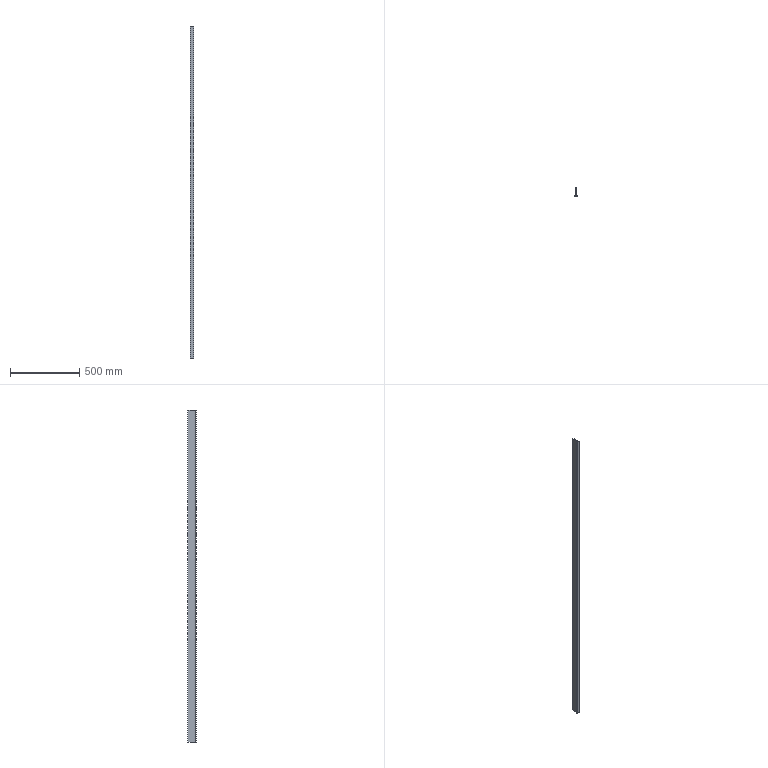Part | SolidWorks | features Fillet 2, Extrusion 1 | 1 solid | 12 faces | box 26 x 60 x 2400 mm | volume 1150265 mm3 | plane 8 | cylinder 4 | commonest cylinder face diameters 10 x2 16 x2
STEP:
#1=CARTESIAN_POINT('',(-3.,30.,0.));
#2=VERTEX_POINT('',#1);
#3=CARTESIAN_POINT('',(-3.,-17.,0.));
#4=VERTEX_POINT('',#3);
#5=CARTESIAN_POINT('',(-3.,30.,0.));
#6=DIRECTION('',(0.,-1.,0.));
#7=VECTOR('',#6,1000.);
#8=LINE('',#5,#7);
#9=EDGE_CURVE('',#2,#4,#8,.T.);
#10=ORIENTED_EDGE('',*,*,#9,.T.);
#11=CARTESIAN_POINT('',(-3.,-17.,2400.));
#12=VERTEX_POINT('',#11);
#13=CARTESIAN_POINT('',(-3.,-17.,2400.));
#14=DIRECTION('',(0.,0.,1.));
#15=VECTOR('',#14,1000.);
#16=LINE('',#13,#15);
#17=EDGE_CURVE('',#4,#12,#16,.T.);
#18=ORIENTED_EDGE('',*,*,#17,.T.);
#19=CARTESIAN_POINT('',(-3.,30.,2400.));
#20=VERTEX_POINT('',#19);
#21=CARTESIAN_POINT('',(-3.,30.,2400.));
#22=DIRECTION('',(0.,-1.,0.));
#23=VECTOR('',#22,1000.);
#24=LINE('',#21,#23);
#25=EDGE_CURVE('',#20,#12,#24,.T.);
#26=ORIENTED_EDGE('',*,*,#25,.F.);
#27=CARTESIAN_POINT('',(-3.,30.,2400.));
#28=DIRECTION('',(0.,0.,-1.));
#29=VECTOR('',#28,1000.);
#30=LINE('',#27,#29);
#31=EDGE_CURVE('',#20,#2,#30,.T.);
#32=ORIENTED_EDGE('',*,*,#31,.T.);
#33=EDGE_LOOP('',(#10,#18,#26,#32));
#34=FACE_OUTER_BOUND('',#33,.T.);
#35=CARTESIAN_POINT('',(-3.,30.,2400.));
#36=DIRECTION('',(1.,0.,0.));
#37=DIRECTION('',(0.,1.,0.));
#38=AXIS2_PLACEMENT_3D('',#35,#36,#37);
#39=PLANE('',#38);
#40=ADVANCED_FACE('',(#34),#39,.F.);
#41=CARTESIAN_POINT('',(-13.,-29.649,2400.));
#42=VERTEX_POINT('',#41);
#43=CARTESIAN_POINT('',(-13.,-30.,2400.));
#44=VERTEX_POINT('',#43);
#45=CARTESIAN_POINT('',(-13.,-25.,2400.));
#46=DIRECTION('',(0.,-1.,0.));
#47=VECTOR('',#46,1000.);
#48=LINE('',#45,#47);
#49=EDGE_CURVE('',#42,#44,#48,.T.);
#50=ORIENTED_EDGE('',*,*,#49,.F.);
#51=CARTESIAN_POINT('',(-13.,-29.649,0.));
#52=VERTEX_POINT('',#51);
#53=CARTESIAN_POINT('',(-13.,-29.649,2400.));
#54=DIRECTION('',(0.,0.,-1.));
#55=VECTOR('',#54,1000.);
#56=LINE('',#53,#55);
#57=EDGE_CURVE('',#42,#52,#56,.T.);
#58=ORIENTED_EDGE('',*,*,#57,.T.);
#59=CARTESIAN_POINT('',(-13.,-30.,0.));
#60=VERTEX_POINT('',#59);
#61=CARTESIAN_POINT('',(-13.,-25.,0.));
#62=DIRECTION('',(0.,-1.,0.));
#63=VECTOR('',#62,1000.);
#64=LINE('',#61,#63);
#65=EDGE_CURVE('',#52,#60,#64,.T.);
#66=ORIENTED_EDGE('',*,*,#65,.T.);
#67=CARTESIAN_POINT('',(-13.,-30.,2400.));
#68=DIRECTION('',(0.,0.,-1.));
#69=VECTOR('',#68,1000.);
#70=LINE('',#67,#69);
#71=EDGE_CURVE('',#44,#60,#70,.T.);
#72=ORIENTED_EDGE('',*,*,#71,.F.);
#73=EDGE_LOOP('',(#50,#58,#66,#72));
#74=FACE_OUTER_BOUND('',#73,.T.);
#75=CARTESIAN_POINT('',(-13.,-25.,2400.));
#76=DIRECTION('',(1.,0.,0.));
#77=DIRECTION('',(0.,0.,-1.));
#78=AXIS2_PLACEMENT_3D('',#75,#76,#77);
#79=PLANE('',#78);
#80=ADVANCED_FACE('',(#74),#79,.F.);
#81=CARTESIAN_POINT('',(13.,-30.,0.));
#82=VERTEX_POINT('',#81);
#83=CARTESIAN_POINT('',(-13.,-30.,0.));
#84=DIRECTION('',(1.,0.,0.));
#85=VECTOR('',#84,1000.);
#86=LINE('',#83,#85);
#87=EDGE_CURVE('',#60,#82,#86,.T.);
#88=ORIENTED_EDGE('',*,*,#87,.T.);
#89=CARTESIAN_POINT('',(13.,-30.,2400.));
#90=VERTEX_POINT('',#89);
#91=CARTESIAN_POINT('',(13.,-30.,2400.));
#92=DIRECTION('',(0.,0.,-1.));
#93=VECTOR('',#92,1000.);
#94=LINE('',#91,#93);
#95=EDGE_CURVE('',#90,#82,#94,.T.);
#96=ORIENTED_EDGE('',*,*,#95,.F.);
#97=CARTESIAN_POINT('',(-13.,-30.,2400.));
#98=DIRECTION('',(1.,0.,0.));
#99=VECTOR('',#98,1000.);
#100=LINE('',#97,#99);
#101=EDGE_CURVE('',#44,#90,#100,.T.);
#102=ORIENTED_EDGE('',*,*,#101,.F.);
#103=ORIENTED_EDGE('',*,*,#71,.T.);
#104=EDGE_LOOP('',(#88,#96,#102,#103));
#105=FACE_OUTER_BOUND('',#104,.T.);
#106=CARTESIAN_POINT('',(-13.,-30.,2400.));
#107=DIRECTION('',(0.,1.,0.));
#108=DIRECTION('',(0.,0.,1.));
#109=AXIS2_PLACEMENT_3D('',#106,#107,#108);
#110=PLANE('',#109);
#111=ADVANCED_FACE('',(#105),#110,.F.);
#112=CARTESIAN_POINT('',(13.,-29.649,0.));
#113=VERTEX_POINT('',#112);
#114=CARTESIAN_POINT('',(13.,-25.,0.));
#115=DIRECTION('',(0.,1.,0.));
#116=VECTOR('',#115,1000.);
#117=LINE('',#114,#116);
#118=EDGE_CURVE('',#82,#113,#117,.T.);
#119=ORIENTED_EDGE('',*,*,#118,.T.);
#120=CARTESIAN_POINT('',(13.,-29.649,2400.));
#121=VERTEX_POINT('',#120);
#122=CARTESIAN_POINT('',(13.,-29.649,2400.));
#123=DIRECTION('',(0.,0.,1.));
#124=VECTOR('',#123,1000.);
#125=LINE('',#122,#124);
#126=EDGE_CURVE('',#113,#121,#125,.T.);
#127=ORIENTED_EDGE('',*,*,#126,.T.);
#128=CARTESIAN_POINT('',(13.,-25.,2400.));
#129=DIRECTION('',(0.,1.,0.));
#130=VECTOR('',#129,1000.);
#131=LINE('',#128,#130);
#132=EDGE_CURVE('',#90,#121,#131,.T.);
#133=ORIENTED_EDGE('',*,*,#132,.F.);
#134=ORIENTED_EDGE('',*,*,#95,.T.);
#135=EDGE_LOOP('',(#119,#127,#133,#134));
#136=FACE_OUTER_BOUND('',#135,.T.);
#137=CARTESIAN_POINT('',(13.,-25.,2400.));
#138=DIRECTION('',(-1.,0.,0.));
#139=DIRECTION('',(0.,0.,1.));
#140=AXIS2_PLACEMENT_3D('',#137,#138,#139);
#141=PLANE('',#140);
#142=ADVANCED_FACE('',(#136),#141,.F.);
#143=CARTESIAN_POINT('',(3.,-17.,2400.));
#144=VERTEX_POINT('',#143);
#145=CARTESIAN_POINT('',(3.,30.,2400.));
#146=VERTEX_POINT('',#145);
#147=CARTESIAN_POINT('',(3.,30.,2400.));
#148=DIRECTION('',(0.,1.,0.));
#149=VECTOR('',#148,1000.);
#150=LINE('',#147,#149);
#151=EDGE_CURVE('',#144,#146,#150,.T.);
#152=ORIENTED_EDGE('',*,*,#151,.F.);
#153=CARTESIAN_POINT('',(3.,-17.,0.));
#154=VERTEX_POINT('',#153);
#155=CARTESIAN_POINT('',(3.,-17.,0.));
#156=DIRECTION('',(0.,0.,-1.));
#157=VECTOR('',#156,1000.);
#158=LINE('',#155,#157);
#159=EDGE_CURVE('',#144,#154,#158,.T.);
#160=ORIENTED_EDGE('',*,*,#159,.T.);
#161=CARTESIAN_POINT('',(3.,30.,0.));
#162=VERTEX_POINT('',#161);
#163=CARTESIAN_POINT('',(3.,30.,0.));
#164=DIRECTION('',(0.,1.,0.));
#165=VECTOR('',#164,1000.);
#166=LINE('',#163,#165);
#167=EDGE_CURVE('',#154,#162,#166,.T.);
#168=ORIENTED_EDGE('',*,*,#167,.T.);
#169=CARTESIAN_POINT('',(3.,30.,2400.));
#170=DIRECTION('',(0.,0.,-1.));
#171=VECTOR('',#170,1000.);
#172=LINE('',#169,#171);
#173=EDGE_CURVE('',#146,#162,#172,.T.);
#174=ORIENTED_EDGE('',*,*,#173,.F.);
#175=EDGE_LOOP('',(#152,#160,#168,#174));
#176=FACE_OUTER_BOUND('',#175,.T.);
#177=CARTESIAN_POINT('',(3.,30.,2400.));
#178=DIRECTION('',(-1.,0.,0.));
#179=DIRECTION('',(0.,-1.,0.));
#180=AXIS2_PLACEMENT_3D('',#177,#178,#179);
#181=PLANE('',#180);
#182=ADVANCED_FACE('',(#176),#181,.F.);
#183=CARTESIAN_POINT('',(-3.,30.,0.));
#184=DIRECTION('',(-1.,0.,0.));
#185=VECTOR('',#184,1000.);
#186=LINE('',#183,#185);
#187=EDGE_CURVE('',#162,#2,#186,.T.);
#188=ORIENTED_EDGE('',*,*,#187,.T.);
#189=ORIENTED_EDGE('',*,*,#31,.F.);
#190=CARTESIAN_POINT('',(-3.,30.,2400.));
#191=DIRECTION('',(-1.,0.,0.));
#192=VECTOR('',#191,1000.);
#193=LINE('',#190,#192);
#194=EDGE_CURVE('',#146,#20,#193,.T.);
#195=ORIENTED_EDGE('',*,*,#194,.F.);
#196=ORIENTED_EDGE('',*,*,#173,.T.);
#197=EDGE_LOOP('',(#188,#189,#195,#196));
#198=FACE_OUTER_BOUND('',#197,.T.);
#199=CARTESIAN_POINT('',(-3.,30.,2400.));
#200=DIRECTION('',(0.,-1.,0.));
#201=DIRECTION('',(0.,0.,-1.));
#202=AXIS2_PLACEMENT_3D('',#199,#200,#201);
#203=PLANE('',#202);
#204=ADVANCED_FACE('',(#198),#203,.F.);
#205=CARTESIAN_POINT('',(-9.154,-24.784,2400.));
#206=VERTEX_POINT('',#205);
#207=CARTESIAN_POINT('',(-11.,-17.,2400.));
#208=DIRECTION('',(0.,0.,-1.));
#209=DIRECTION('',(-1.,0.,0.));
#210=AXIS2_PLACEMENT_3D('',#207,#208,#209);
#211=CIRCLE('',#210,8.);
#212=EDGE_CURVE('',#12,#206,#211,.T.);
#213=ORIENTED_EDGE('',*,*,#212,.T.);
#214=CARTESIAN_POINT('',(-8.,-29.649,2400.));
#215=DIRECTION('',(0.,0.,1.));
#216=DIRECTION('',(-1.,0.,0.));
#217=AXIS2_PLACEMENT_3D('',#214,#215,#216);
#218=CIRCLE('',#217,5.);
#219=EDGE_CURVE('',#206,#42,#218,.T.);
#220=ORIENTED_EDGE('',*,*,#219,.T.);
#221=ORIENTED_EDGE('',*,*,#49,.T.);
#222=ORIENTED_EDGE('',*,*,#101,.T.);
#223=ORIENTED_EDGE('',*,*,#132,.T.);
#224=CARTESIAN_POINT('',(9.154,-24.784,2400.));
#225=VERTEX_POINT('',#224);
#226=CARTESIAN_POINT('',(8.,-29.649,2400.));
#227=DIRECTION('',(0.,0.,1.));
#228=DIRECTION('',(-1.,0.,0.));
#229=AXIS2_PLACEMENT_3D('',#226,#227,#228);
#230=CIRCLE('',#229,5.);
#231=EDGE_CURVE('',#121,#225,#230,.T.);
#232=ORIENTED_EDGE('',*,*,#231,.T.);
#233=CARTESIAN_POINT('',(11.,-17.,2400.));
#234=DIRECTION('',(0.,0.,-1.));
#235=DIRECTION('',(-1.,0.,0.));
#236=AXIS2_PLACEMENT_3D('',#233,#234,#235);
#237=CIRCLE('',#236,8.);
#238=EDGE_CURVE('',#225,#144,#237,.T.);
#239=ORIENTED_EDGE('',*,*,#238,.T.);
#240=ORIENTED_EDGE('',*,*,#151,.T.);
#241=ORIENTED_EDGE('',*,*,#194,.T.);
#242=ORIENTED_EDGE('',*,*,#25,.T.);
#243=EDGE_LOOP('',(#213,#220,#221,#222,#223,#232,#239,#240,#241,#242));
#244=FACE_OUTER_BOUND('',#243,.T.);
#245=CARTESIAN_POINT('',(-3.,-25.,2400.));
#246=DIRECTION('',(0.,0.,-1.));
#247=DIRECTION('',(-1.,0.,0.));
#248=AXIS2_PLACEMENT_3D('',#245,#246,#247);
#249=PLANE('',#248);
#250=ADVANCED_FACE('',(#244),#249,.F.);
#251=ORIENTED_EDGE('',*,*,#65,.F.);
#252=CARTESIAN_POINT('',(-9.154,-24.784,0.));
#253=VERTEX_POINT('',#252);
#254=CARTESIAN_POINT('',(-8.,-29.649,0.));
#255=DIRECTION('',(0.,0.,-1.));
#256=DIRECTION('',(-1.,0.,0.));
#257=AXIS2_PLACEMENT_3D('',#254,#255,#256);
#258=CIRCLE('',#257,5.);
#259=EDGE_CURVE('',#52,#253,#258,.T.);
#260=ORIENTED_EDGE('',*,*,#259,.T.);
#261=CARTESIAN_POINT('',(-11.,-17.,0.));
#262=DIRECTION('',(0.,0.,1.));
#263=DIRECTION('',(-1.,0.,0.));
#264=AXIS2_PLACEMENT_3D('',#261,#262,#263);
#265=CIRCLE('',#264,8.);
#266=EDGE_CURVE('',#253,#4,#265,.T.);
#267=ORIENTED_EDGE('',*,*,#266,.T.);
#268=ORIENTED_EDGE('',*,*,#9,.F.);
#269=ORIENTED_EDGE('',*,*,#187,.F.);
#270=ORIENTED_EDGE('',*,*,#167,.F.);
#271=CARTESIAN_POINT('',(9.154,-24.784,0.));
#272=VERTEX_POINT('',#271);
#273=CARTESIAN_POINT('',(11.,-17.,0.));
#274=DIRECTION('',(0.,0.,1.));
#275=DIRECTION('',(-1.,0.,0.));
#276=AXIS2_PLACEMENT_3D('',#273,#274,#275);
#277=CIRCLE('',#276,8.);
#278=EDGE_CURVE('',#154,#272,#277,.T.);
#279=ORIENTED_EDGE('',*,*,#278,.T.);
#280=CARTESIAN_POINT('',(8.,-29.649,0.));
#281=DIRECTION('',(0.,0.,-1.));
#282=DIRECTION('',(-1.,0.,0.));
#283=AXIS2_PLACEMENT_3D('',#280,#281,#282);
#284=CIRCLE('',#283,5.);
#285=EDGE_CURVE('',#272,#113,#284,.T.);
#286=ORIENTED_EDGE('',*,*,#285,.T.);
#287=ORIENTED_EDGE('',*,*,#118,.F.);
#288=ORIENTED_EDGE('',*,*,#87,.F.);
#289=EDGE_LOOP('',(#251,#260,#267,#268,#269,#270,#279,#286,#287,#288));
#290=FACE_OUTER_BOUND('',#289,.T.);
#291=CARTESIAN_POINT('',(-3.,-25.,0.));
#292=DIRECTION('',(0.,0.,-1.));
#293=DIRECTION('',(-1.,0.,0.));
#294=AXIS2_PLACEMENT_3D('',#291,#292,#293);
#295=PLANE('',#294);
#296=ADVANCED_FACE('',(#290),#295,.T.);
#297=ORIENTED_EDGE('',*,*,#266,.F.);
#298=CARTESIAN_POINT('',(-9.154,-24.784,2400.));
#299=DIRECTION('',(0.,0.,1.));
#300=VECTOR('',#299,1000.);
#301=LINE('',#298,#300);
#302=EDGE_CURVE('',#253,#206,#301,.T.);
#303=ORIENTED_EDGE('',*,*,#302,.T.);
#304=ORIENTED_EDGE('',*,*,#212,.F.);
#305=ORIENTED_EDGE('',*,*,#17,.F.);
#306=EDGE_LOOP('',(#297,#303,#304,#305));
#307=FACE_OUTER_BOUND('',#306,.T.);
#308=CARTESIAN_POINT('',(-11.,-17.,2400.));
#309=DIRECTION('',(0.,0.,1.));
#310=DIRECTION('',(1.,0.,0.));
#311=AXIS2_PLACEMENT_3D('',#308,#309,#310);
#312=CYLINDRICAL_SURFACE('',#311,8.);
#313=ADVANCED_FACE('',(#307),#312,.F.);
#314=ORIENTED_EDGE('',*,*,#238,.F.);
#315=CARTESIAN_POINT('',(9.154,-24.784,2400.));
#316=DIRECTION('',(0.,0.,-1.));
#317=VECTOR('',#316,1000.);
#318=LINE('',#315,#317);
#319=EDGE_CURVE('',#225,#272,#318,.T.);
#320=ORIENTED_EDGE('',*,*,#319,.T.);
#321=ORIENTED_EDGE('',*,*,#278,.F.);
#322=ORIENTED_EDGE('',*,*,#159,.F.);
#323=EDGE_LOOP('',(#314,#320,#321,#322));
#324=FACE_OUTER_BOUND('',#323,.T.);
#325=CARTESIAN_POINT('',(11.,-17.,2400.));
#326=DIRECTION('',(0.,0.,1.));
#327=DIRECTION('',(1.,0.,0.));
#328=AXIS2_PLACEMENT_3D('',#325,#326,#327);
#329=CYLINDRICAL_SURFACE('',#328,8.);
#330=ADVANCED_FACE('',(#324),#329,.F.);
#331=ORIENTED_EDGE('',*,*,#219,.F.);
#332=ORIENTED_EDGE('',*,*,#302,.F.);
#333=ORIENTED_EDGE('',*,*,#259,.F.);
#334=ORIENTED_EDGE('',*,*,#57,.F.);
#335=EDGE_LOOP('',(#331,#332,#333,#334));
#336=FACE_OUTER_BOUND('',#335,.T.);
#337=CARTESIAN_POINT('',(-8.,-29.649,2400.));
#338=DIRECTION('',(0.,0.,1.));
#339=DIRECTION('',(1.,0.,0.));
#340=AXIS2_PLACEMENT_3D('',#337,#338,#339);
#341=CYLINDRICAL_SURFACE('',#340,5.);
#342=ADVANCED_FACE('',(#336),#341,.T.);
#343=ORIENTED_EDGE('',*,*,#231,.F.);
#344=ORIENTED_EDGE('',*,*,#126,.F.);
#345=ORIENTED_EDGE('',*,*,#285,.F.);
#346=ORIENTED_EDGE('',*,*,#319,.F.);
#347=EDGE_LOOP('',(#343,#344,#345,#346));
#348=FACE_OUTER_BOUND('',#347,.T.);
#349=CARTESIAN_POINT('',(8.,-29.649,2400.));
#350=DIRECTION('',(0.,0.,1.));
#351=DIRECTION('',(1.,0.,0.));
#352=AXIS2_PLACEMENT_3D('',#349,#350,#351);
#353=CYLINDRICAL_SURFACE('',#352,5.);
#354=ADVANCED_FACE('',(#348),#353,.T.);
#355=CLOSED_SHELL('',(#40,#80,#111,#142,#182,#204,#250,#296,#313,#330,#342,#354));
#356=MANIFOLD_SOLID_BREP('',#355);
#357=CARTESIAN_POINT('',(0.,0.,0.));
#358=DIRECTION('',(0.,0.,1.));
#359=DIRECTION('',(1.,0.,0.));
#360=AXIS2_PLACEMENT_3D('',#357,#358,#359);
#361=(LENGTH_UNIT()NAMED_UNIT(*)SI_UNIT(.MILLI.,.METRE.));
#362=UNCERTAINTY_MEASURE_WITH_UNIT(LENGTH_MEASURE(0.00001),#361,'','');
#363=(NAMED_UNIT(*)PLANE_ANGLE_UNIT()SI_UNIT($,.RADIAN.));
#364=(NAMED_UNIT(*)SI_UNIT($,.STERADIAN.)SOLID_ANGLE_UNIT());
#365=(GEOMETRIC_REPRESENTATION_CONTEXT(3)GLOBAL_UNCERTAINTY_ASSIGNED_CONTEXT((#362))GLOBAL_UNIT_ASSIGNED_CONTEXT((#361,#363,#364))REPRESENTATION_CONTEXT('',''));
#366=ADVANCED_BREP_SHAPE_REPRESENTATION('',(#356,#360),#365);